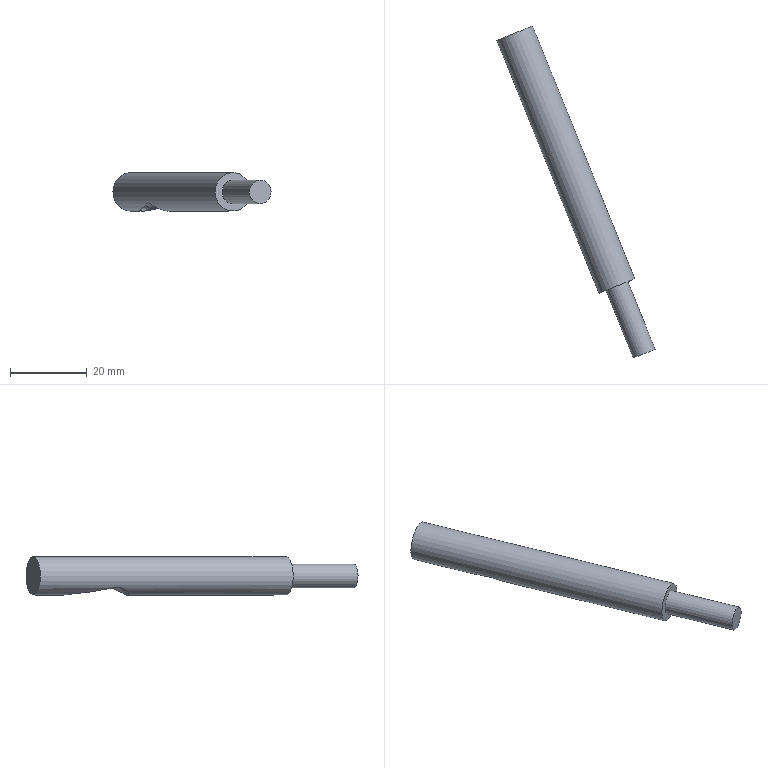Part | NX | features solid 2 | 1 solid | 8 faces | volume 5884 mm3 | plane 3 | cylinder 2 | sphere 2 | cone 1 | commonest cylinder face diameters 6.1 x1 10 x1
STEP:
#1=CARTESIAN_POINT('',(-689.979,331.032,95.108));
#2=VERTEX_POINT('',#1);
#3=CARTESIAN_POINT('',(-696.498,340.532,93.42));
#4=VERTEX_POINT('',#3);
#5=CARTESIAN_POINT('',(-689.979,331.032,95.108));
#6=CARTESIAN_POINT('',(-691.996,334.248,94.267));
#7=CARTESIAN_POINT('',(-694.217,337.396,93.702));
#8=CARTESIAN_POINT('',(-696.498,340.532,93.42));
#9=B_SPLINE_CURVE_WITH_KNOTS('',3,(#5,#6,#7,#8),.UNSPECIFIED.,.F.,.F.,(4,4),(0.000000208,0.01165),.UNSPECIFIED.);
#10=EDGE_CURVE('',#2,#4,#9,.T.);
#11=ORIENTED_EDGE('',*,*,#10,.T.);
#12=CARTESIAN_POINT('',(-699.162,339.456,93.42));
#13=VERTEX_POINT('',#12);
#14=CARTESIAN_POINT('',(-696.498,340.532,93.42));
#15=CARTESIAN_POINT('',(-696.888,341.07,93.372));
#16=CARTESIAN_POINT('',(-698.43,341.483,93.047));
#17=CARTESIAN_POINT('',(-699.254,340.114,93.372));
#18=CARTESIAN_POINT('',(-699.162,339.456,93.42));
#19=B_SPLINE_CURVE_WITH_KNOTS('',3,(#14,#15,#16,#17,#18),.UNSPECIFIED.,.F.,.F.,(4,1,4),(0.000000204,0.001971,0.003941),.UNSPECIFIED.);
#20=EDGE_CURVE('',#4,#13,#19,.T.);
#21=ORIENTED_EDGE('',*,*,#20,.T.);
#22=CARTESIAN_POINT('',(-697.252,328.094,95.108));
#23=VERTEX_POINT('',#22);
#24=CARTESIAN_POINT('',(-699.162,339.456,93.42));
#25=CARTESIAN_POINT('',(-698.625,335.614,93.703));
#26=CARTESIAN_POINT('',(-698.036,331.811,94.266));
#27=CARTESIAN_POINT('',(-697.252,328.094,95.108));
#28=B_SPLINE_CURVE_WITH_KNOTS('',3,(#24,#25,#26,#27),.UNSPECIFIED.,.F.,.F.,(4,4),(0.000000207,0.01167),.UNSPECIFIED.);
#29=EDGE_CURVE('',#13,#23,#28,.T.);
#30=ORIENTED_EDGE('',*,*,#29,.T.);
#31=CARTESIAN_POINT('',(-697.252,328.094,95.108));
#32=CARTESIAN_POINT('',(-697.111,327.427,95.259));
#33=CARTESIAN_POINT('',(-696.597,326.103,95.285));
#34=CARTESIAN_POINT('',(-695.319,324.576,94.504));
#35=CARTESIAN_POINT('',(-693.553,323.881,93.523));
#36=CARTESIAN_POINT('',(-691.46,324.19,93.054));
#37=CARTESIAN_POINT('',(-689.718,325.421,93.517));
#38=CARTESIAN_POINT('',(-688.926,327.159,94.504));
#39=CARTESIAN_POINT('',(-689.065,329.137,95.283));
#40=CARTESIAN_POINT('',(-689.617,330.454,95.259));
#41=CARTESIAN_POINT('',(-689.979,331.032,95.108));
#42=B_SPLINE_CURVE_WITH_KNOTS('',3,(#31,#32,#33,#34,#35,#36,#37,#38,#39,#40,#41),.UNSPECIFIED.,.F.,.F.,(4,1,1,1,1,1,1,1,4),(0.000000205,0.002065,0.00413,0.006195,0.00826,0.01033,0.01239,0.01446,0.01652),.UNSPECIFIED.);
#43=EDGE_CURVE('',#23,#2,#42,.T.);
#44=ORIENTED_EDGE('',*,*,#43,.T.);
#45=EDGE_LOOP('',(#11,#21,#30,#44));
#46=FACE_BOUND('',#45,.T.);
#47=CARTESIAN_POINT('',(-696.8,350.791,98.209));
#48=VERTEX_POINT('',#47);
#49=CARTESIAN_POINT('',(-701.435,348.918,98.209));
#50=DIRECTION('',(-0.3746,0.9272,0.));
#51=DIRECTION('',(0.9272,0.3746,0.));
#52=AXIS2_PLACEMENT_3D('',#49,#50,#51);
#53=CIRCLE('',#52,5.);
#54=EDGE_CURVE('',#48,#48,#53,.T.);
#55=ORIENTED_EDGE('',*,*,#54,.F.);
#56=EDGE_LOOP('',(#55));
#57=FACE_BOUND('',#56,.T.);
#58=CARTESIAN_POINT('',(-670.202,284.961,98.209));
#59=VERTEX_POINT('',#58);
#60=CARTESIAN_POINT('',(-674.838,283.088,98.209));
#61=DIRECTION('',(-0.3746,0.9272,0.));
#62=DIRECTION('',(0.9272,0.3746,0.));
#63=AXIS2_PLACEMENT_3D('',#60,#61,#62);
#64=CIRCLE('',#63,5.);
#65=EDGE_CURVE('',#59,#59,#64,.T.);
#66=ORIENTED_EDGE('',*,*,#65,.T.);
#67=EDGE_LOOP('',(#66));
#68=FACE_BOUND('',#67,.T.);
#69=CARTESIAN_POINT('',(-701.435,348.918,98.209));
#70=DIRECTION('',(0.3746,-0.9272,0.));
#71=DIRECTION('',(-0.9272,-0.3746,0.));
#72=AXIS2_PLACEMENT_3D('',#69,#70,#71);
#73=CYLINDRICAL_SURFACE('',#72,5.);
#74=ADVANCED_FACE('',(#46,#57,#68),#73,.T.);
#75=ORIENTED_EDGE('',*,*,#54,.T.);
#76=EDGE_LOOP('',(#75));
#77=FACE_BOUND('',#76,.T.);
#78=CARTESIAN_POINT('',(-701.435,348.918,98.209));
#79=DIRECTION('',(-0.3746,0.9272,0.));
#80=DIRECTION('',(0.9272,0.3746,0.));
#81=AXIS2_PLACEMENT_3D('',#78,#79,#80);
#82=PLANE('',#81);
#83=ADVANCED_FACE('',(#77),#82,.T.);
#84=CARTESIAN_POINT('',(-672.01,284.23,98.209));
#85=VERTEX_POINT('',#84);
#86=CARTESIAN_POINT('',(-674.838,283.088,98.209));
#87=DIRECTION('',(-0.3746,0.9272,0.));
#88=DIRECTION('',(0.9272,0.3746,0.));
#89=AXIS2_PLACEMENT_3D('',#86,#87,#88);
#90=CIRCLE('',#89,3.05);
#91=EDGE_CURVE('',#85,#85,#90,.T.);
#92=ORIENTED_EDGE('',*,*,#91,.T.);
#93=EDGE_LOOP('',(#92));
#94=FACE_BOUND('',#93,.T.);
#95=ORIENTED_EDGE('',*,*,#65,.F.);
#96=EDGE_LOOP('',(#95));
#97=FACE_BOUND('',#96,.T.);
#98=CARTESIAN_POINT('',(-674.838,283.088,98.209));
#99=DIRECTION('',(-0.3746,0.9272,0.));
#100=DIRECTION('',(0.9272,0.3746,0.));
#101=AXIS2_PLACEMENT_3D('',#98,#99,#100);
#102=PLANE('',#101);
#103=ADVANCED_FACE('',(#94,#97),#102,.F.);
#104=CARTESIAN_POINT('',(-664.893,266.614,98.209));
#105=VERTEX_POINT('',#104);
#106=CARTESIAN_POINT('',(-667.721,265.471,98.209));
#107=DIRECTION('',(-0.3746,0.9272,0.));
#108=DIRECTION('',(0.9272,0.3746,0.));
#109=AXIS2_PLACEMENT_3D('',#106,#107,#108);
#110=CIRCLE('',#109,3.05);
#111=EDGE_CURVE('',#105,#105,#110,.T.);
#112=ORIENTED_EDGE('',*,*,#111,.T.);
#113=EDGE_LOOP('',(#112));
#114=FACE_BOUND('',#113,.T.);
#115=ORIENTED_EDGE('',*,*,#91,.F.);
#116=EDGE_LOOP('',(#115));
#117=FACE_BOUND('',#116,.T.);
#118=CARTESIAN_POINT('',(-667.721,265.471,98.209));
#119=DIRECTION('',(-0.3746,0.9272,0.));
#120=DIRECTION('',(0.9272,0.3746,0.));
#121=AXIS2_PLACEMENT_3D('',#118,#119,#120);
#122=CYLINDRICAL_SURFACE('',#121,3.05);
#123=ADVANCED_FACE('',(#114,#117),#122,.T.);
#124=ORIENTED_EDGE('',*,*,#111,.F.);
#125=EDGE_LOOP('',(#124));
#126=FACE_BOUND('',#125,.T.);
#127=CARTESIAN_POINT('',(-667.721,265.471,98.209));
#128=DIRECTION('',(-0.3746,0.9272,0.));
#129=DIRECTION('',(0.9272,0.3746,0.));
#130=AXIS2_PLACEMENT_3D('',#127,#128,#129);
#131=PLANE('',#130);
#132=ADVANCED_FACE('',(#126),#131,.F.);
#133=CARTESIAN_POINT('',(-693.616,329.563,93.209));
#134=DIRECTION('',(0.3746,-0.9272,0.));
#135=DIRECTION('',(-0.9272,-0.3746,0.));
#136=AXIS2_PLACEMENT_3D('',#133,#134,#135);
#137=CIRCLE('',#136,4.357);
#138=EDGE_CURVE('',#2,#23,#137,.T.);
#139=ORIENTED_EDGE('',*,*,#138,.F.);
#140=ORIENTED_EDGE('',*,*,#43,.F.);
#141=EDGE_LOOP('',(#139,#140));
#142=FACE_BOUND('',#141,.T.);
#143=CARTESIAN_POINT('',(-693.194,328.52,93.209));
#144=DIRECTION('',(0.3746,-0.9272,0.));
#145=DIRECTION('',(-0.9272,-0.3746,0.));
#146=AXIS2_PLACEMENT_3D('',#143,#144,#145);
#147=SPHERICAL_SURFACE('',#146,4.5);
#148=ADVANCED_FACE('',(#142),#147,.F.);
#149=CARTESIAN_POINT('',(-697.83,339.994,93.209));
#150=DIRECTION('',(0.3746,-0.9272,0.));
#151=DIRECTION('',(-0.9272,-0.3746,0.));
#152=AXIS2_PLACEMENT_3D('',#149,#150,#151);
#153=CIRCLE('',#152,1.452);
#154=EDGE_CURVE('',#4,#13,#153,.T.);
#155=ORIENTED_EDGE('',*,*,#154,.F.);
#156=ORIENTED_EDGE('',*,*,#10,.F.);
#157=ORIENTED_EDGE('',*,*,#138,.T.);
#158=ORIENTED_EDGE('',*,*,#29,.F.);
#159=EDGE_LOOP('',(#155,#156,#157,#158));
#160=FACE_BOUND('',#159,.T.);
#161=CARTESIAN_POINT('',(-693.616,329.563,93.209));
#162=DIRECTION('',(0.3746,-0.9272,0.));
#163=DIRECTION('',(-0.9272,-0.3746,0.));
#164=AXIS2_PLACEMENT_3D('',#161,#162,#163);
#165=CONICAL_SURFACE('',#164,4.357,0.2527);
#166=ADVANCED_FACE('',(#160),#165,.F.);
#167=ORIENTED_EDGE('',*,*,#154,.T.);
#168=ORIENTED_EDGE('',*,*,#20,.F.);
#169=EDGE_LOOP('',(#167,#168));
#170=FACE_BOUND('',#169,.T.);
#171=CARTESIAN_POINT('',(-697.689,339.646,93.209));
#172=DIRECTION('',(0.3746,-0.9272,0.));
#173=DIRECTION('',(0.9272,0.3746,0.));
#174=AXIS2_PLACEMENT_3D('',#171,#172,#173);
#175=SPHERICAL_SURFACE('',#174,1.5);
#176=ADVANCED_FACE('',(#170),#175,.F.);
#177=CLOSED_SHELL('',(#74,#83,#103,#123,#132,#148,#166,#176));
#178=MANIFOLD_SOLID_BREP('',#177);
#179=(LENGTH_UNIT()NAMED_UNIT(*)SI_UNIT(.MILLI.,.METRE.));
#180=UNCERTAINTY_MEASURE_WITH_UNIT(LENGTH_MEASURE(0.0508),#179,'','');
#181=(NAMED_UNIT(*)PLANE_ANGLE_UNIT()SI_UNIT($,.RADIAN.));
#182=(NAMED_UNIT(*)SI_UNIT($,.STERADIAN.)SOLID_ANGLE_UNIT());
#183=(GEOMETRIC_REPRESENTATION_CONTEXT(3)GLOBAL_UNCERTAINTY_ASSIGNED_CONTEXT((#180))GLOBAL_UNIT_ASSIGNED_CONTEXT((#179,#181,#182))REPRESENTATION_CONTEXT('',''));
#184=ADVANCED_BREP_SHAPE_REPRESENTATION('',(#178),#183);